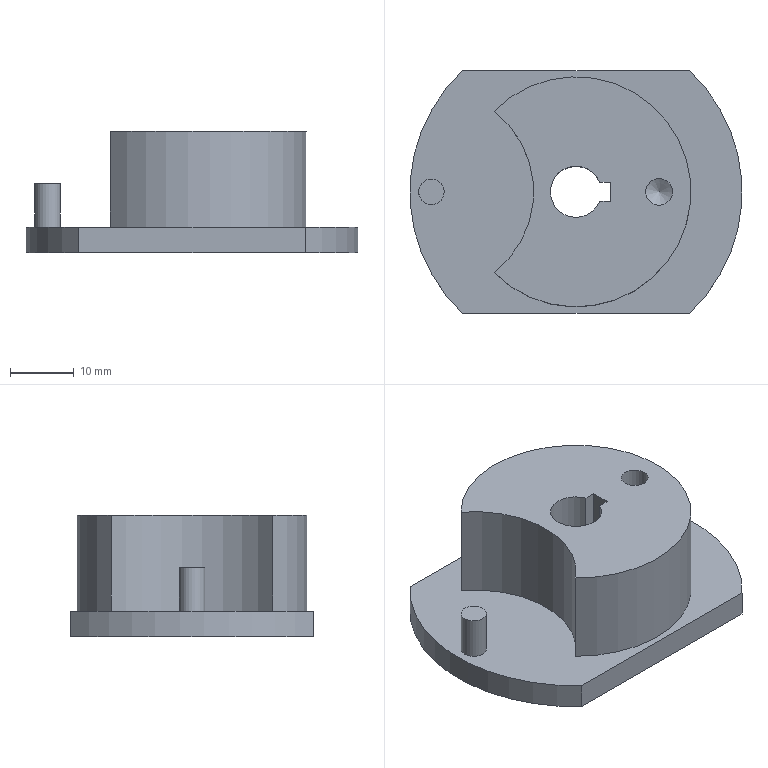Part | NX | features BREP 1, DATUM_CSYS 1 | 1 solid | 18 faces | box 52 x 38 x 19 mm | volume 18337 mm3 | plane 9 | cylinder 6 | spline 2 | cone 1 | commonest cylinder face diameters 4.2 x2 52 x2 4 x1 8 x1
STEP:
#1=CARTESIAN_POINT('',(-17.748,-19.,-4.));
#2=VERTEX_POINT('',#1);
#3=CARTESIAN_POINT('',(17.748,-19.,-4.));
#4=VERTEX_POINT('',#3);
#5=CARTESIAN_POINT('',(-17.748,-19.,-4.));
#6=DIRECTION('',(1.,0.,0.));
#7=VECTOR('',#6,1000.);
#8=LINE('',#5,#7);
#9=EDGE_CURVE('',#2,#4,#8,.T.);
#10=ORIENTED_EDGE('',*,*,#9,.F.);
#11=CARTESIAN_POINT('',(-17.748,19.,-4.));
#12=VERTEX_POINT('',#11);
#13=CARTESIAN_POINT('',(0.,0.,-4.));
#14=DIRECTION('',(0.,0.,-1.));
#15=DIRECTION('',(-0.6826,-0.7308,0.));
#16=AXIS2_PLACEMENT_3D('',#13,#14,#15);
#17=CIRCLE('',#16,26.);
#18=EDGE_CURVE('',#2,#12,#17,.T.);
#19=ORIENTED_EDGE('',*,*,#18,.T.);
#20=CARTESIAN_POINT('',(17.748,19.,-4.));
#21=VERTEX_POINT('',#20);
#22=CARTESIAN_POINT('',(17.748,19.,-4.));
#23=DIRECTION('',(-1.,0.,0.));
#24=VECTOR('',#23,1000.);
#25=LINE('',#22,#24);
#26=EDGE_CURVE('',#21,#12,#25,.T.);
#27=ORIENTED_EDGE('',*,*,#26,.F.);
#28=CARTESIAN_POINT('',(0.,0.,-4.));
#29=DIRECTION('',(0.,0.,1.));
#30=DIRECTION('',(0.6826,-0.7308,0.));
#31=AXIS2_PLACEMENT_3D('',#28,#29,#30);
#32=CIRCLE('',#31,26.);
#33=EDGE_CURVE('',#4,#21,#32,.T.);
#34=ORIENTED_EDGE('',*,*,#33,.F.);
#35=EDGE_LOOP('',(#10,#19,#27,#34));
#36=FACE_BOUND('',#35,.T.);
#37=CARTESIAN_POINT('',(5.4,1.5,-4.));
#38=VERTEX_POINT('',#37);
#39=CARTESIAN_POINT('',(5.4,-1.5,-4.));
#40=VERTEX_POINT('',#39);
#41=CARTESIAN_POINT('',(5.4,1.5,-4.));
#42=DIRECTION('',(0.,-1.,0.));
#43=VECTOR('',#42,1000.);
#44=LINE('',#41,#43);
#45=EDGE_CURVE('',#38,#40,#44,.T.);
#46=ORIENTED_EDGE('',*,*,#45,.F.);
#47=CARTESIAN_POINT('',(3.708,1.5,-4.));
#48=VERTEX_POINT('',#47);
#49=CARTESIAN_POINT('',(3.708,1.5,-4.));
#50=DIRECTION('',(1.,0.,0.));
#51=VECTOR('',#50,1000.);
#52=LINE('',#49,#51);
#53=EDGE_CURVE('',#48,#38,#52,.T.);
#54=ORIENTED_EDGE('',*,*,#53,.F.);
#55=CARTESIAN_POINT('',(3.708,-1.5,-4.));
#56=VERTEX_POINT('',#55);
#57=CARTESIAN_POINT('',(0.,0.,-4.));
#58=DIRECTION('',(0.,0.,-1.));
#59=DIRECTION('',(0.927,-0.375,0.));
#60=AXIS2_PLACEMENT_3D('',#57,#58,#59);
#61=CIRCLE('',#60,4.);
#62=EDGE_CURVE('',#56,#48,#61,.T.);
#63=ORIENTED_EDGE('',*,*,#62,.F.);
#64=CARTESIAN_POINT('',(5.4,-1.5,-4.));
#65=DIRECTION('',(-1.,0.,0.));
#66=VECTOR('',#65,1000.);
#67=LINE('',#64,#66);
#68=EDGE_CURVE('',#40,#56,#67,.T.);
#69=ORIENTED_EDGE('',*,*,#68,.F.);
#70=EDGE_LOOP('',(#46,#54,#63,#69));
#71=FACE_BOUND('',#70,.T.);
#72=CARTESIAN_POINT('',(0.,0.,-4.));
#73=DIRECTION('',(0.,0.,-1.));
#74=DIRECTION('',(-1.,0.,0.));
#75=AXIS2_PLACEMENT_3D('',#72,#73,#74);
#76=PLANE('',#75);
#77=ADVANCED_FACE('',(#36,#71),#76,.T.);
#78=CARTESIAN_POINT('',(-17.748,-19.,0.));
#79=VERTEX_POINT('',#78);
#80=CARTESIAN_POINT('',(-17.748,19.,0.));
#81=VERTEX_POINT('',#80);
#82=CARTESIAN_POINT('',(0.,0.,0.));
#83=DIRECTION('',(0.,0.,-1.));
#84=DIRECTION('',(-0.6826,-0.7308,0.));
#85=AXIS2_PLACEMENT_3D('',#82,#83,#84);
#86=CIRCLE('',#85,26.);
#87=EDGE_CURVE('',#79,#81,#86,.T.);
#88=ORIENTED_EDGE('',*,*,#87,.F.);
#89=CARTESIAN_POINT('',(17.748,-19.,0.));
#90=VERTEX_POINT('',#89);
#91=CARTESIAN_POINT('',(17.748,-19.,0.));
#92=DIRECTION('',(-1.,0.,0.));
#93=VECTOR('',#92,1000.);
#94=LINE('',#91,#93);
#95=EDGE_CURVE('',#90,#79,#94,.T.);
#96=ORIENTED_EDGE('',*,*,#95,.F.);
#97=CARTESIAN_POINT('',(17.748,19.,0.));
#98=VERTEX_POINT('',#97);
#99=CARTESIAN_POINT('',(0.,0.,0.));
#100=DIRECTION('',(0.,0.,1.));
#101=DIRECTION('',(0.6826,-0.7308,0.));
#102=AXIS2_PLACEMENT_3D('',#99,#100,#101);
#103=CIRCLE('',#102,26.);
#104=EDGE_CURVE('',#90,#98,#103,.T.);
#105=ORIENTED_EDGE('',*,*,#104,.T.);
#106=CARTESIAN_POINT('',(-17.748,19.,0.));
#107=DIRECTION('',(1.,0.,0.));
#108=VECTOR('',#107,1000.);
#109=LINE('',#106,#108);
#110=EDGE_CURVE('',#81,#98,#109,.T.);
#111=ORIENTED_EDGE('',*,*,#110,.F.);
#112=EDGE_LOOP('',(#88,#96,#105,#111));
#113=FACE_BOUND('',#112,.T.);
#114=CARTESIAN_POINT('',(-12.816,12.639,0.));
#115=VERTEX_POINT('',#114);
#116=CARTESIAN_POINT('',(-12.816,-12.639,0.));
#117=VERTEX_POINT('',#116);
#118=CARTESIAN_POINT('',(-22.627,0.,0.));
#119=DIRECTION('',(0.,0.,-1.));
#120=DIRECTION('',(0.6132,0.7899,0.));
#121=AXIS2_PLACEMENT_3D('',#118,#119,#120);
#122=CIRCLE('',#121,16.);
#123=EDGE_CURVE('',#115,#117,#122,.T.);
#124=ORIENTED_EDGE('',*,*,#123,.F.);
#125=CARTESIAN_POINT('',(0.,0.,0.));
#126=DIRECTION('',(0.,0.,-1.));
#127=DIRECTION('',(-0.712,0.7022,0.));
#128=AXIS2_PLACEMENT_3D('',#125,#126,#127);
#129=CIRCLE('',#128,18.);
#130=EDGE_CURVE('',#115,#117,#129,.T.);
#131=ORIENTED_EDGE('',*,*,#130,.T.);
#132=EDGE_LOOP('',(#124,#131));
#133=FACE_BOUND('',#132,.T.);
#134=CARTESIAN_POINT('',(-20.627,0.,0.));
#135=VERTEX_POINT('',#134);
#136=CARTESIAN_POINT('',(-22.627,0.,0.));
#137=DIRECTION('',(0.,0.,1.));
#138=DIRECTION('',(1.,0.,0.));
#139=AXIS2_PLACEMENT_3D('',#136,#137,#138);
#140=CIRCLE('',#139,2.);
#141=EDGE_CURVE('',#135,#135,#140,.T.);
#142=ORIENTED_EDGE('',*,*,#141,.F.);
#143=EDGE_LOOP('',(#142));
#144=FACE_BOUND('',#143,.T.);
#145=CARTESIAN_POINT('',(-9.199,0.,0.));
#146=DIRECTION('',(0.,0.,-1.));
#147=DIRECTION('',(-1.,0.,0.));
#148=AXIS2_PLACEMENT_3D('',#145,#146,#147);
#149=PLANE('',#148);
#150=ADVANCED_FACE('',(#113,#133,#144),#149,.F.);
#151=ORIENTED_EDGE('',*,*,#141,.T.);
#152=CARTESIAN_POINT('',(-20.627,0.,6.8));
#153=VERTEX_POINT('',#152);
#154=CARTESIAN_POINT('',(-20.627,0.,0.));
#155=DIRECTION('',(0.,0.,1.));
#156=VECTOR('',#155,1000.);
#157=LINE('',#154,#156);
#158=EDGE_CURVE('',#135,#153,#157,.T.);
#159=ORIENTED_EDGE('',*,*,#158,.T.);
#160=CARTESIAN_POINT('',(-22.627,0.,6.8));
#161=DIRECTION('',(0.,0.,1.));
#162=DIRECTION('',(1.,0.,0.));
#163=AXIS2_PLACEMENT_3D('',#160,#161,#162);
#164=CIRCLE('',#163,2.);
#165=EDGE_CURVE('',#153,#153,#164,.T.);
#166=ORIENTED_EDGE('',*,*,#165,.F.);
#167=ORIENTED_EDGE('',*,*,#158,.F.);
#168=EDGE_LOOP('',(#151,#159,#166,#167));
#169=FACE_BOUND('',#168,.T.);
#170=CARTESIAN_POINT('',(-22.627,0.,0.));
#171=DIRECTION('',(0.,0.,1.));
#172=DIRECTION('',(-1.,0.,0.));
#173=AXIS2_PLACEMENT_3D('',#170,#171,#172);
#174=CYLINDRICAL_SURFACE('',#173,2.);
#175=ADVANCED_FACE('',(#169),#174,.T.);
#176=CARTESIAN_POINT('',(-12.816,-12.639,15.));
#177=VERTEX_POINT('',#176);
#178=CARTESIAN_POINT('',(-12.816,-12.639,0.));
#179=DIRECTION('',(0.,0.,1.));
#180=VECTOR('',#179,1000.);
#181=LINE('',#178,#180);
#182=EDGE_CURVE('',#117,#177,#181,.T.);
#183=ORIENTED_EDGE('',*,*,#182,.F.);
#184=ORIENTED_EDGE('',*,*,#130,.F.);
#185=CARTESIAN_POINT('',(-12.816,12.639,15.));
#186=VERTEX_POINT('',#185);
#187=CARTESIAN_POINT('',(-12.816,12.639,15.));
#188=DIRECTION('',(0.,0.,-1.));
#189=VECTOR('',#188,1000.);
#190=LINE('',#187,#189);
#191=EDGE_CURVE('',#186,#115,#190,.T.);
#192=ORIENTED_EDGE('',*,*,#191,.F.);
#193=CARTESIAN_POINT('',(0.,0.,15.));
#194=DIRECTION('',(0.,0.,-1.));
#195=DIRECTION('',(-0.712,0.7022,0.));
#196=AXIS2_PLACEMENT_3D('',#193,#194,#195);
#197=CIRCLE('',#196,18.);
#198=EDGE_CURVE('',#186,#177,#197,.T.);
#199=ORIENTED_EDGE('',*,*,#198,.T.);
#200=EDGE_LOOP('',(#183,#184,#192,#199));
#201=FACE_BOUND('',#200,.T.);
#202=CARTESIAN_POINT('',(-12.816,-12.639,0.));
#203=CARTESIAN_POINT('',(-12.816,-12.639,15.));
#204=CARTESIAN_POINT('',(-11.108,-14.372,0.));
#205=CARTESIAN_POINT('',(-11.108,-14.372,15.));
#206=CARTESIAN_POINT('',(-9.,-15.588,0.));
#207=CARTESIAN_POINT('',(-9.,-15.588,15.));
#208=CARTESIAN_POINT('',(18.,-31.177,0.));
#209=CARTESIAN_POINT('',(18.,-31.177,15.));
#210=CARTESIAN_POINT('',(18.,0.,0.));
#211=CARTESIAN_POINT('',(18.,0.,15.));
#212=CARTESIAN_POINT('',(18.,31.177,0.));
#213=CARTESIAN_POINT('',(18.,31.177,15.));
#214=CARTESIAN_POINT('',(-9.,15.588,0.));
#215=CARTESIAN_POINT('',(-9.,15.588,15.));
#216=CARTESIAN_POINT('',(-11.108,14.372,0.));
#217=CARTESIAN_POINT('',(-11.108,14.372,15.));
#218=CARTESIAN_POINT('',(-12.816,12.639,0.));
#219=CARTESIAN_POINT('',(-12.816,12.639,15.));
#220=(BOUNDED_SURFACE()B_SPLINE_SURFACE(2,1,((#202,#203),(#204,#205),(#206,#207),(#208,#209),(#210,#211),(#212,#213),(#214,#215),(#216,#217),(#218,#219)),.SURF_OF_LINEAR_EXTRUSION.,.F.,.F.,.F.)B_SPLINE_SURFACE_WITH_KNOTS((3,2,2,2,3),(2,2),(0.06859,0.1275,0.5343,0.9411,1.),(0.,0.6522),.PIECEWISE_BEZIER_KNOTS.)GEOMETRIC_REPRESENTATION_ITEM()RATIONAL_B_SPLINE_SURFACE(((0.8762,0.8762),(0.9276,0.9276),(1.,1.),(0.5,0.5),(1.,1.),(0.5,0.5),(1.,1.),(0.9276,0.9276),(0.8762,0.8762)))REPRESENTATION_ITEM('')SURFACE());
#221=ADVANCED_FACE('',(#201),#220,.T.);
#222=ORIENTED_EDGE('',*,*,#165,.T.);
#223=EDGE_LOOP('',(#222));
#224=FACE_BOUND('',#223,.T.);
#225=CARTESIAN_POINT('',(-23.163,0.,6.8));
#226=DIRECTION('',(0.,0.,1.));
#227=DIRECTION('',(-1.,0.,0.));
#228=AXIS2_PLACEMENT_3D('',#225,#226,#227);
#229=PLANE('',#228);
#230=ADVANCED_FACE('',(#224),#229,.T.);
#231=CARTESIAN_POINT('',(-22.627,0.,15.));
#232=DIRECTION('',(0.,0.,-1.));
#233=DIRECTION('',(0.6132,0.7899,0.));
#234=AXIS2_PLACEMENT_3D('',#231,#232,#233);
#235=CIRCLE('',#234,16.);
#236=EDGE_CURVE('',#186,#177,#235,.T.);
#237=ORIENTED_EDGE('',*,*,#236,.T.);
#238=ORIENTED_EDGE('',*,*,#198,.F.);
#239=EDGE_LOOP('',(#237,#238));
#240=FACE_BOUND('',#239,.T.);
#241=CARTESIAN_POINT('',(3.708,-1.5,15.));
#242=VERTEX_POINT('',#241);
#243=CARTESIAN_POINT('',(3.708,1.5,15.));
#244=VERTEX_POINT('',#243);
#245=CARTESIAN_POINT('',(0.,0.,15.));
#246=DIRECTION('',(0.,0.,-1.));
#247=DIRECTION('',(0.927,-0.375,0.));
#248=AXIS2_PLACEMENT_3D('',#245,#246,#247);
#249=CIRCLE('',#248,4.);
#250=EDGE_CURVE('',#242,#244,#249,.T.);
#251=ORIENTED_EDGE('',*,*,#250,.T.);
#252=CARTESIAN_POINT('',(5.4,1.5,15.));
#253=VERTEX_POINT('',#252);
#254=CARTESIAN_POINT('',(5.4,1.5,15.));
#255=DIRECTION('',(-1.,0.,0.));
#256=VECTOR('',#255,1000.);
#257=LINE('',#254,#256);
#258=EDGE_CURVE('',#253,#244,#257,.T.);
#259=ORIENTED_EDGE('',*,*,#258,.F.);
#260=CARTESIAN_POINT('',(5.4,-1.5,15.));
#261=VERTEX_POINT('',#260);
#262=CARTESIAN_POINT('',(5.4,-1.5,15.));
#263=DIRECTION('',(0.,1.,0.));
#264=VECTOR('',#263,1000.);
#265=LINE('',#262,#264);
#266=EDGE_CURVE('',#261,#253,#265,.T.);
#267=ORIENTED_EDGE('',*,*,#266,.F.);
#268=CARTESIAN_POINT('',(3.708,-1.5,15.));
#269=DIRECTION('',(1.,0.,0.));
#270=VECTOR('',#269,1000.);
#271=LINE('',#268,#270);
#272=EDGE_CURVE('',#242,#261,#271,.T.);
#273=ORIENTED_EDGE('',*,*,#272,.F.);
#274=EDGE_LOOP('',(#251,#259,#267,#273));
#275=FACE_BOUND('',#274,.T.);
#276=CARTESIAN_POINT('',(15.1,0.,15.));
#277=VERTEX_POINT('',#276);
#278=CARTESIAN_POINT('',(13.,0.,15.));
#279=DIRECTION('',(0.,0.,-1.));
#280=DIRECTION('',(1.,0.,0.));
#281=AXIS2_PLACEMENT_3D('',#278,#279,#280);
#282=CIRCLE('',#281,2.1);
#283=EDGE_CURVE('',#277,#277,#282,.T.);
#284=ORIENTED_EDGE('',*,*,#283,.T.);
#285=EDGE_LOOP('',(#284));
#286=FACE_BOUND('',#285,.T.);
#287=CARTESIAN_POINT('',(-4.823,0.,15.));
#288=DIRECTION('',(0.,0.,1.));
#289=DIRECTION('',(-1.,0.,0.));
#290=AXIS2_PLACEMENT_3D('',#287,#288,#289);
#291=PLANE('',#290);
#292=ADVANCED_FACE('',(#240,#275,#286),#291,.T.);
#293=CARTESIAN_POINT('',(17.748,19.,0.));
#294=DIRECTION('',(0.,0.,-1.));
#295=VECTOR('',#294,1000.);
#296=LINE('',#293,#295);
#297=EDGE_CURVE('',#98,#21,#296,.T.);
#298=ORIENTED_EDGE('',*,*,#297,.F.);
#299=ORIENTED_EDGE('',*,*,#104,.F.);
#300=CARTESIAN_POINT('',(17.748,-19.,-4.));
#301=DIRECTION('',(0.,0.,1.));
#302=VECTOR('',#301,1000.);
#303=LINE('',#300,#302);
#304=EDGE_CURVE('',#4,#90,#303,.T.);
#305=ORIENTED_EDGE('',*,*,#304,.F.);
#306=ORIENTED_EDGE('',*,*,#33,.T.);
#307=EDGE_LOOP('',(#298,#299,#305,#306));
#308=FACE_BOUND('',#307,.T.);
#309=CARTESIAN_POINT('',(0.,0.,0.));
#310=DIRECTION('',(0.,0.,-1.));
#311=DIRECTION('',(-0.6826,-0.7308,0.));
#312=AXIS2_PLACEMENT_3D('',#309,#310,#311);
#313=CYLINDRICAL_SURFACE('',#312,26.);
#314=ADVANCED_FACE('',(#308),#313,.T.);
#315=ORIENTED_EDGE('',*,*,#87,.T.);
#316=CARTESIAN_POINT('',(-17.748,19.,-4.));
#317=DIRECTION('',(0.,0.,1.));
#318=VECTOR('',#317,1000.);
#319=LINE('',#316,#318);
#320=EDGE_CURVE('',#12,#81,#319,.T.);
#321=ORIENTED_EDGE('',*,*,#320,.F.);
#322=ORIENTED_EDGE('',*,*,#18,.F.);
#323=CARTESIAN_POINT('',(-17.748,-19.,0.));
#324=DIRECTION('',(0.,0.,-1.));
#325=VECTOR('',#324,1000.);
#326=LINE('',#323,#325);
#327=EDGE_CURVE('',#79,#2,#326,.T.);
#328=ORIENTED_EDGE('',*,*,#327,.F.);
#329=EDGE_LOOP('',(#315,#321,#322,#328));
#330=FACE_BOUND('',#329,.T.);
#331=CARTESIAN_POINT('',(0.,0.,0.));
#332=DIRECTION('',(0.,0.,-1.));
#333=DIRECTION('',(-1.,0.,0.));
#334=AXIS2_PLACEMENT_3D('',#331,#332,#333);
#335=CYLINDRICAL_SURFACE('',#334,26.);
#336=ADVANCED_FACE('',(#330),#335,.T.);
#337=ORIENTED_EDGE('',*,*,#95,.T.);
#338=ORIENTED_EDGE('',*,*,#327,.T.);
#339=ORIENTED_EDGE('',*,*,#9,.T.);
#340=ORIENTED_EDGE('',*,*,#304,.T.);
#341=EDGE_LOOP('',(#337,#338,#339,#340));
#342=FACE_BOUND('',#341,.T.);
#343=CARTESIAN_POINT('',(0.,-19.,-18.5));
#344=DIRECTION('',(0.,-1.,0.));
#345=DIRECTION('',(1.,0.,0.));
#346=AXIS2_PLACEMENT_3D('',#343,#344,#345);
#347=PLANE('',#346);
#348=ADVANCED_FACE('',(#342),#347,.T.);
#349=ORIENTED_EDGE('',*,*,#110,.T.);
#350=ORIENTED_EDGE('',*,*,#297,.T.);
#351=ORIENTED_EDGE('',*,*,#26,.T.);
#352=ORIENTED_EDGE('',*,*,#320,.T.);
#353=EDGE_LOOP('',(#349,#350,#351,#352));
#354=FACE_BOUND('',#353,.T.);
#355=CARTESIAN_POINT('',(0.,19.,-18.5));
#356=DIRECTION('',(0.,1.,0.));
#357=DIRECTION('',(-1.,0.,0.));
#358=AXIS2_PLACEMENT_3D('',#355,#356,#357);
#359=PLANE('',#358);
#360=ADVANCED_FACE('',(#354),#359,.T.);
#361=ORIENTED_EDGE('',*,*,#182,.T.);
#362=ORIENTED_EDGE('',*,*,#236,.F.);
#363=ORIENTED_EDGE('',*,*,#191,.T.);
#364=ORIENTED_EDGE('',*,*,#123,.T.);
#365=EDGE_LOOP('',(#361,#362,#363,#364));
#366=FACE_BOUND('',#365,.T.);
#367=CARTESIAN_POINT('',(-12.816,-12.639,15.));
#368=CARTESIAN_POINT('',(-12.816,-12.639,0.));
#369=CARTESIAN_POINT('',(-6.627,-7.835,15.));
#370=CARTESIAN_POINT('',(-6.627,-7.835,0.));
#371=CARTESIAN_POINT('',(-6.627,0.,15.));
#372=CARTESIAN_POINT('',(-6.627,0.,0.));
#373=CARTESIAN_POINT('',(-6.627,7.835,15.));
#374=CARTESIAN_POINT('',(-6.627,7.835,0.));
#375=CARTESIAN_POINT('',(-12.816,12.639,15.));
#376=CARTESIAN_POINT('',(-12.816,12.639,0.));
#377=(BOUNDED_SURFACE()B_SPLINE_SURFACE(2,1,((#367,#368),(#369,#370),(#371,#372),(#373,#374),(#375,#376)),.SURF_OF_LINEAR_EXTRUSION.,.F.,.F.,.F.)B_SPLINE_SURFACE_WITH_KNOTS((3,2,3),(2,2),(0.1562,0.5781,1.),(0.1176,1.),.PIECEWISE_BEZIER_KNOTS.)GEOMETRIC_REPRESENTATION_ITEM()RATIONAL_B_SPLINE_SURFACE(((0.7535,0.7535),(0.7796,0.7796),(1.,1.),(0.7796,0.7796),(0.7535,0.7535)))REPRESENTATION_ITEM('')SURFACE());
#378=ADVANCED_FACE('',(#366),#377,.T.);
#379=ORIENTED_EDGE('',*,*,#62,.T.);
#380=CARTESIAN_POINT('',(3.708,1.5,15.));
#381=DIRECTION('',(0.,0.,-1.));
#382=VECTOR('',#381,1000.);
#383=LINE('',#380,#382);
#384=EDGE_CURVE('',#244,#48,#383,.T.);
#385=ORIENTED_EDGE('',*,*,#384,.F.);
#386=ORIENTED_EDGE('',*,*,#250,.F.);
#387=CARTESIAN_POINT('',(3.708,-1.5,-4.));
#388=DIRECTION('',(0.,0.,1.));
#389=VECTOR('',#388,1000.);
#390=LINE('',#387,#389);
#391=EDGE_CURVE('',#56,#242,#390,.T.);
#392=ORIENTED_EDGE('',*,*,#391,.F.);
#393=EDGE_LOOP('',(#379,#385,#386,#392));
#394=FACE_BOUND('',#393,.T.);
#395=CARTESIAN_POINT('',(0.,0.,15.));
#396=DIRECTION('',(0.,0.,-1.));
#397=DIRECTION('',(-1.,0.,0.));
#398=AXIS2_PLACEMENT_3D('',#395,#396,#397);
#399=CYLINDRICAL_SURFACE('',#398,4.);
#400=ADVANCED_FACE('',(#394),#399,.F.);
#401=ORIENTED_EDGE('',*,*,#266,.T.);
#402=CARTESIAN_POINT('',(5.4,1.5,15.));
#403=DIRECTION('',(0.,0.,-1.));
#404=VECTOR('',#403,1000.);
#405=LINE('',#402,#404);
#406=EDGE_CURVE('',#253,#38,#405,.T.);
#407=ORIENTED_EDGE('',*,*,#406,.T.);
#408=ORIENTED_EDGE('',*,*,#45,.T.);
#409=CARTESIAN_POINT('',(5.4,-1.5,15.));
#410=DIRECTION('',(0.,0.,-1.));
#411=VECTOR('',#410,1000.);
#412=LINE('',#409,#411);
#413=EDGE_CURVE('',#261,#40,#412,.T.);
#414=ORIENTED_EDGE('',*,*,#413,.F.);
#415=EDGE_LOOP('',(#401,#407,#408,#414));
#416=FACE_BOUND('',#415,.T.);
#417=CARTESIAN_POINT('',(5.4,3.,-25.8));
#418=DIRECTION('',(-1.,0.,0.));
#419=DIRECTION('',(0.,-1.,0.));
#420=AXIS2_PLACEMENT_3D('',#417,#418,#419);
#421=PLANE('',#420);
#422=ADVANCED_FACE('',(#416),#421,.T.);
#423=ORIENTED_EDGE('',*,*,#258,.T.);
#424=ORIENTED_EDGE('',*,*,#384,.T.);
#425=ORIENTED_EDGE('',*,*,#53,.T.);
#426=ORIENTED_EDGE('',*,*,#406,.F.);
#427=EDGE_LOOP('',(#423,#424,#425,#426));
#428=FACE_BOUND('',#427,.T.);
#429=CARTESIAN_POINT('',(3.594,1.5,-25.8));
#430=DIRECTION('',(0.,-1.,0.));
#431=DIRECTION('',(1.,0.,0.));
#432=AXIS2_PLACEMENT_3D('',#429,#430,#431);
#433=PLANE('',#432);
#434=ADVANCED_FACE('',(#428),#433,.T.);
#435=ORIENTED_EDGE('',*,*,#413,.T.);
#436=ORIENTED_EDGE('',*,*,#68,.T.);
#437=ORIENTED_EDGE('',*,*,#391,.T.);
#438=ORIENTED_EDGE('',*,*,#272,.T.);
#439=EDGE_LOOP('',(#435,#436,#437,#438));
#440=FACE_BOUND('',#439,.T.);
#441=CARTESIAN_POINT('',(3.594,-1.5,-25.8));
#442=DIRECTION('',(0.,1.,0.));
#443=DIRECTION('',(-1.,0.,0.));
#444=AXIS2_PLACEMENT_3D('',#441,#442,#443);
#445=PLANE('',#444);
#446=ADVANCED_FACE('',(#440),#445,.T.);
#447=CARTESIAN_POINT('',(15.1,0.,5.));
#448=VERTEX_POINT('',#447);
#449=CARTESIAN_POINT('',(15.1,0.,15.));
#450=DIRECTION('',(0.,0.,-1.));
#451=VECTOR('',#450,1000.);
#452=LINE('',#449,#451);
#453=EDGE_CURVE('',#277,#448,#452,.T.);
#454=ORIENTED_EDGE('',*,*,#453,.T.);
#455=CARTESIAN_POINT('',(13.,0.,5.));
#456=DIRECTION('',(0.,0.,-1.));
#457=DIRECTION('',(1.,0.,0.));
#458=AXIS2_PLACEMENT_3D('',#455,#456,#457);
#459=CIRCLE('',#458,2.1);
#460=EDGE_CURVE('',#448,#448,#459,.T.);
#461=ORIENTED_EDGE('',*,*,#460,.T.);
#462=ORIENTED_EDGE('',*,*,#453,.F.);
#463=ORIENTED_EDGE('',*,*,#283,.F.);
#464=EDGE_LOOP('',(#454,#461,#462,#463));
#465=FACE_BOUND('',#464,.T.);
#466=CARTESIAN_POINT('',(13.,0.,15.));
#467=DIRECTION('',(0.,0.,-1.));
#468=DIRECTION('',(-1.,0.,0.));
#469=AXIS2_PLACEMENT_3D('',#466,#467,#468);
#470=CYLINDRICAL_SURFACE('',#469,2.1);
#471=ADVANCED_FACE('',(#465),#470,.F.);
#472=CARTESIAN_POINT('',(15.1,0.,3.));
#473=VERTEX_POINT('',#472);
#474=CARTESIAN_POINT('',(15.1,0.,5.));
#475=DIRECTION('',(0.,0.,-1.));
#476=VECTOR('',#475,1000.);
#477=LINE('',#474,#476);
#478=EDGE_CURVE('',#448,#473,#477,.T.);
#479=ORIENTED_EDGE('',*,*,#478,.T.);
#480=CARTESIAN_POINT('',(13.,0.,3.));
#481=DIRECTION('',(0.,0.,-1.));
#482=DIRECTION('',(1.,0.,0.));
#483=AXIS2_PLACEMENT_3D('',#480,#481,#482);
#484=CIRCLE('',#483,2.1);
#485=EDGE_CURVE('',#473,#473,#484,.T.);
#486=ORIENTED_EDGE('',*,*,#485,.T.);
#487=ORIENTED_EDGE('',*,*,#478,.F.);
#488=ORIENTED_EDGE('',*,*,#460,.F.);
#489=EDGE_LOOP('',(#479,#486,#487,#488));
#490=FACE_BOUND('',#489,.T.);
#491=CARTESIAN_POINT('',(13.,0.,5.));
#492=DIRECTION('',(0.,0.,-1.));
#493=DIRECTION('',(-1.,0.,0.));
#494=AXIS2_PLACEMENT_3D('',#491,#492,#493);
#495=CYLINDRICAL_SURFACE('',#494,2.1);
#496=ADVANCED_FACE('',(#490),#495,.F.);
#497=CARTESIAN_POINT('',(13.,0.,1.738));
#498=VERTEX_POINT('',#497);
#499=CARTESIAN_POINT('',(15.1,0.,3.));
#500=DIRECTION('',(-0.8572,0.,-0.515));
#501=VECTOR('',#500,1000.);
#502=LINE('',#499,#501);
#503=EDGE_CURVE('',#473,#498,#502,.T.);
#504=ORIENTED_EDGE('',*,*,#503,.T.);
#505=ORIENTED_EDGE('',*,*,#503,.F.);
#506=ORIENTED_EDGE('',*,*,#485,.F.);
#507=EDGE_LOOP('',(#504,#505,#506));
#508=FACE_BOUND('',#507,.T.);
#509=CARTESIAN_POINT('',(13.,0.,1.738));
#510=DIRECTION('',(0.,0.,1.));
#511=DIRECTION('',(-1.,0.,0.));
#512=AXIS2_PLACEMENT_3D('',#509,#510,#511);
#513=CONICAL_SURFACE('',#512,0.,1.03);
#514=ADVANCED_FACE('',(#508),#513,.F.);
#515=CLOSED_SHELL('',(#77,#150,#175,#221,#230,#292,#314,#336,#348,#360,#378,#400,#422,#434,#446,#471,#496,#514));
#516=MANIFOLD_SOLID_BREP('',#515);
#517=(LENGTH_UNIT()NAMED_UNIT(*)SI_UNIT(.MILLI.,.METRE.));
#518=UNCERTAINTY_MEASURE_WITH_UNIT(LENGTH_MEASURE(0.00001),#517,'','');
#519=(NAMED_UNIT(*)PLANE_ANGLE_UNIT()SI_UNIT($,.RADIAN.));
#520=(NAMED_UNIT(*)SI_UNIT($,.STERADIAN.)SOLID_ANGLE_UNIT());
#521=(GEOMETRIC_REPRESENTATION_CONTEXT(3)GLOBAL_UNCERTAINTY_ASSIGNED_CONTEXT((#518))GLOBAL_UNIT_ASSIGNED_CONTEXT((#517,#519,#520))REPRESENTATION_CONTEXT('',''));
#522=ADVANCED_BREP_SHAPE_REPRESENTATION('',(#516),#521);